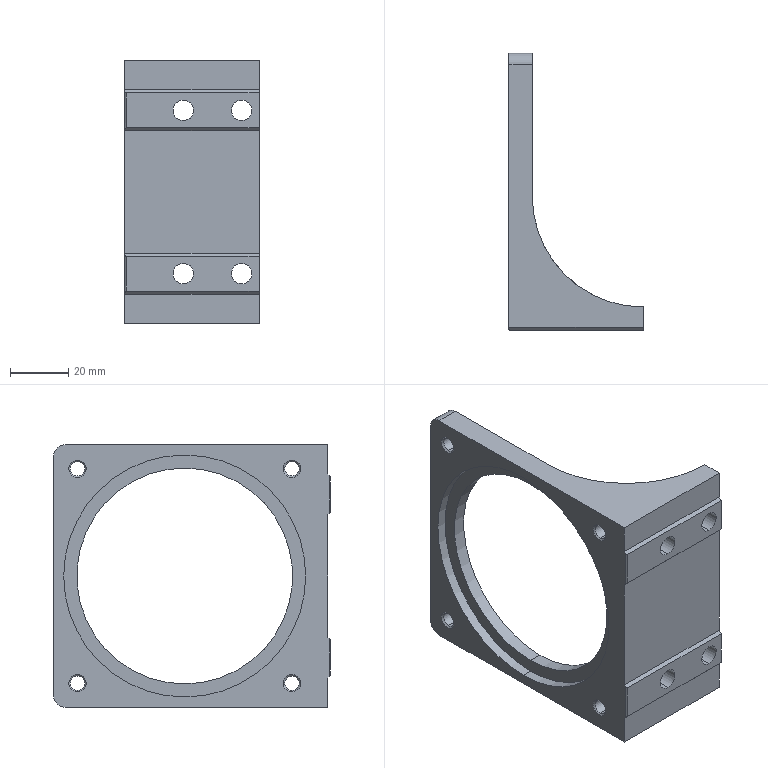Part | STEP file | 0230_Z_013_PACMR90-W40-V100-MTB90_2 | 1 solid | 68 faces | box 46 x 95 x 90 mm | volume 55942 mm3 | cylinder 29 | plane 23 | cone 16 | commonest cylinder face diameters 4.917 x8 7 x8 8.4 x3 1 x2 8 x2 74 x2